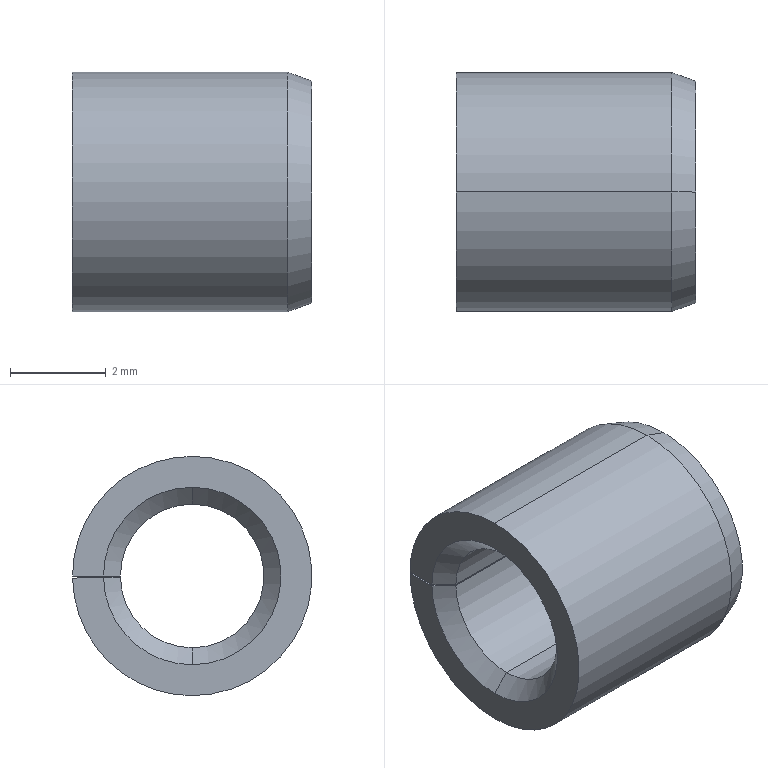Part | SolidWorks | features MBimport 1 | 1 solid | 19 faces | box 5 x 5 x 5 mm | volume 60.695 mm3 | cone 9 | cylinder 6 | plane 4 | commonest cylinder face diameters 3 x3 5 x3
STEP:
#1=CARTESIAN_POINT('',(4.5,0.,2.5));
#2=VERTEX_POINT('',#1);
#3=CARTESIAN_POINT('',(4.5,0.,-2.5));
#4=VERTEX_POINT('',#3);
#5=CARTESIAN_POINT('',(4.5,0.,0.));
#6=DIRECTION('',(1.,0.,0.));
#7=DIRECTION('',(0.,0.,-1.));
#8=AXIS2_PLACEMENT_3D('',#5,#6,#7);
#9=CIRCLE('',#8,2.5);
#10=EDGE_CURVE('',#2,#4,#9,.T.);
#11=ORIENTED_EDGE('',*,*,#10,.F.);
#12=CARTESIAN_POINT('',(0.,0.,2.5));
#13=VERTEX_POINT('',#12);
#14=CARTESIAN_POINT('',(50.,0.,2.5));
#15=DIRECTION('',(-1.,0.,0.));
#16=VECTOR('',#15,1000.);
#17=LINE('',#14,#16);
#18=EDGE_CURVE('',#2,#13,#17,.T.);
#19=ORIENTED_EDGE('',*,*,#18,.T.);
#20=CARTESIAN_POINT('',(0.,0.,-2.5));
#21=VERTEX_POINT('',#20);
#22=CARTESIAN_POINT('',(0.,0.,0.));
#23=DIRECTION('',(1.,0.,0.));
#24=DIRECTION('',(0.,0.,-1.));
#25=AXIS2_PLACEMENT_3D('',#22,#23,#24);
#26=CIRCLE('',#25,2.5);
#27=EDGE_CURVE('',#13,#21,#26,.T.);
#28=ORIENTED_EDGE('',*,*,#27,.T.);
#29=CARTESIAN_POINT('',(50.,0.,-2.5));
#30=DIRECTION('',(-1.,0.,0.));
#31=VECTOR('',#30,1000.);
#32=LINE('',#29,#31);
#33=EDGE_CURVE('',#4,#21,#32,.T.);
#34=ORIENTED_EDGE('',*,*,#33,.F.);
#35=EDGE_LOOP('',(#11,#19,#28,#34));
#36=FACE_OUTER_BOUND('',#35,.T.);
#37=CARTESIAN_POINT('',(50.,0.,0.));
#38=DIRECTION('',(-1.,0.,0.));
#39=DIRECTION('',(0.,0.,-1.));
#40=AXIS2_PLACEMENT_3D('',#37,#38,#39);
#41=CYLINDRICAL_SURFACE('',#40,2.5);
#42=ADVANCED_FACE('',(#36),#41,.T.);
#43=CARTESIAN_POINT('',(4.5,2.5,-0.04363));
#44=VERTEX_POINT('',#43);
#45=CARTESIAN_POINT('',(4.5,0.,0.));
#46=DIRECTION('',(1.,0.,0.));
#47=DIRECTION('',(0.,0.,-1.));
#48=AXIS2_PLACEMENT_3D('',#45,#46,#47);
#49=CIRCLE('',#48,2.5);
#50=EDGE_CURVE('',#4,#44,#49,.T.);
#51=ORIENTED_EDGE('',*,*,#50,.F.);
#52=ORIENTED_EDGE('',*,*,#33,.T.);
#53=CARTESIAN_POINT('',(0.,2.5,-0.04363));
#54=VERTEX_POINT('',#53);
#55=CARTESIAN_POINT('',(0.,0.,0.));
#56=DIRECTION('',(1.,0.,0.));
#57=DIRECTION('',(0.,0.,-1.));
#58=AXIS2_PLACEMENT_3D('',#55,#56,#57);
#59=CIRCLE('',#58,2.5);
#60=EDGE_CURVE('',#21,#54,#59,.T.);
#61=ORIENTED_EDGE('',*,*,#60,.T.);
#62=CARTESIAN_POINT('',(4.5,2.5,-0.04363));
#63=DIRECTION('',(-1.,0.,0.));
#64=VECTOR('',#63,1000.);
#65=LINE('',#62,#64);
#66=EDGE_CURVE('',#44,#54,#65,.T.);
#67=ORIENTED_EDGE('',*,*,#66,.F.);
#68=EDGE_LOOP('',(#51,#52,#61,#67));
#69=FACE_OUTER_BOUND('',#68,.T.);
#70=CARTESIAN_POINT('',(50.,0.,0.));
#71=DIRECTION('',(-1.,0.,0.));
#72=DIRECTION('',(0.,0.,-1.));
#73=AXIS2_PLACEMENT_3D('',#70,#71,#72);
#74=CYLINDRICAL_SURFACE('',#73,2.5);
#75=ADVANCED_FACE('',(#69),#74,.T.);
#76=CARTESIAN_POINT('',(5.,0.,-2.318));
#77=VERTEX_POINT('',#76);
#78=CARTESIAN_POINT('',(5.,2.318,-0.04045));
#79=VERTEX_POINT('',#78);
#80=CARTESIAN_POINT('',(5.,0.,0.));
#81=DIRECTION('',(1.,0.,0.));
#82=DIRECTION('',(0.,0.,-1.));
#83=AXIS2_PLACEMENT_3D('',#80,#81,#82);
#84=CIRCLE('',#83,2.318);
#85=EDGE_CURVE('',#77,#79,#84,.T.);
#86=ORIENTED_EDGE('',*,*,#85,.F.);
#87=CARTESIAN_POINT('',(5.,0.,-2.318));
#88=DIRECTION('',(-0.9397,0.,-0.342));
#89=VECTOR('',#88,1000.);
#90=LINE('',#87,#89);
#91=EDGE_CURVE('',#77,#4,#90,.T.);
#92=ORIENTED_EDGE('',*,*,#91,.T.);
#93=ORIENTED_EDGE('',*,*,#50,.T.);
#94=CARTESIAN_POINT('',(5.,2.318,-0.04045));
#95=DIRECTION('',(-0.9397,0.342,-0.005969));
#96=VECTOR('',#95,1000.);
#97=LINE('',#94,#96);
#98=EDGE_CURVE('',#79,#44,#97,.T.);
#99=ORIENTED_EDGE('',*,*,#98,.F.);
#100=EDGE_LOOP('',(#86,#92,#93,#99));
#101=FACE_OUTER_BOUND('',#100,.T.);
#102=CARTESIAN_POINT('',(5.,0.,0.));
#103=DIRECTION('',(-1.,0.,0.));
#104=DIRECTION('',(0.,0.,1.));
#105=AXIS2_PLACEMENT_3D('',#102,#103,#104);
#106=CONICAL_SURFACE('',#105,2.318,0.3491);
#107=ADVANCED_FACE('',(#101),#106,.T.);
#108=ORIENTED_EDGE('',*,*,#91,.F.);
#109=CARTESIAN_POINT('',(5.,0.,2.318));
#110=VERTEX_POINT('',#109);
#111=CARTESIAN_POINT('',(5.,0.,0.));
#112=DIRECTION('',(1.,0.,0.));
#113=DIRECTION('',(0.,0.,-1.));
#114=AXIS2_PLACEMENT_3D('',#111,#112,#113);
#115=CIRCLE('',#114,2.318);
#116=EDGE_CURVE('',#110,#77,#115,.T.);
#117=ORIENTED_EDGE('',*,*,#116,.F.);
#118=CARTESIAN_POINT('',(5.,0.,2.318));
#119=DIRECTION('',(-0.9397,0.,0.342));
#120=VECTOR('',#119,1000.);
#121=LINE('',#118,#120);
#122=EDGE_CURVE('',#110,#2,#121,.T.);
#123=ORIENTED_EDGE('',*,*,#122,.T.);
#124=ORIENTED_EDGE('',*,*,#10,.T.);
#125=EDGE_LOOP('',(#108,#117,#123,#124));
#126=FACE_OUTER_BOUND('',#125,.T.);
#127=CARTESIAN_POINT('',(5.,0.,0.));
#128=DIRECTION('',(-1.,0.,0.));
#129=DIRECTION('',(0.,0.,1.));
#130=AXIS2_PLACEMENT_3D('',#127,#128,#129);
#131=CONICAL_SURFACE('',#130,2.318,0.3491);
#132=ADVANCED_FACE('',(#126),#131,.T.);
#133=CARTESIAN_POINT('',(0.3536,0.,1.5));
#134=VERTEX_POINT('',#133);
#135=CARTESIAN_POINT('',(0.3536,0.,-1.5));
#136=VERTEX_POINT('',#135);
#137=CARTESIAN_POINT('',(0.3536,0.,0.));
#138=DIRECTION('',(1.,0.,0.));
#139=DIRECTION('',(0.,0.,-1.));
#140=AXIS2_PLACEMENT_3D('',#137,#138,#139);
#141=CIRCLE('',#140,1.5);
#142=EDGE_CURVE('',#134,#136,#141,.T.);
#143=ORIENTED_EDGE('',*,*,#142,.T.);
#144=CARTESIAN_POINT('',(0.,0.,-1.854));
#145=VERTEX_POINT('',#144);
#146=CARTESIAN_POINT('',(0.,0.,-1.854));
#147=DIRECTION('',(-0.7071,0.,-0.7071));
#148=VECTOR('',#147,1000.);
#149=LINE('',#146,#148);
#150=EDGE_CURVE('',#136,#145,#149,.T.);
#151=ORIENTED_EDGE('',*,*,#150,.T.);
#152=CARTESIAN_POINT('',(0.,0.,1.854));
#153=VERTEX_POINT('',#152);
#154=CARTESIAN_POINT('',(0.,0.,0.));
#155=DIRECTION('',(1.,0.,0.));
#156=DIRECTION('',(0.,0.,-1.));
#157=AXIS2_PLACEMENT_3D('',#154,#155,#156);
#158=CIRCLE('',#157,1.854);
#159=EDGE_CURVE('',#153,#145,#158,.T.);
#160=ORIENTED_EDGE('',*,*,#159,.F.);
#161=CARTESIAN_POINT('',(0.,0.,1.854));
#162=DIRECTION('',(-0.7071,0.,0.7071));
#163=VECTOR('',#162,1000.);
#164=LINE('',#161,#163);
#165=EDGE_CURVE('',#134,#153,#164,.T.);
#166=ORIENTED_EDGE('',*,*,#165,.F.);
#167=EDGE_LOOP('',(#143,#151,#160,#166));
#168=FACE_OUTER_BOUND('',#167,.T.);
#169=CARTESIAN_POINT('',(0.,0.,0.));
#170=DIRECTION('',(-1.,0.,0.));
#171=DIRECTION('',(0.,0.,1.));
#172=AXIS2_PLACEMENT_3D('',#169,#170,#171);
#173=CONICAL_SURFACE('',#172,1.854,0.7854);
#174=ADVANCED_FACE('',(#168),#173,.F.);
#175=CARTESIAN_POINT('',(0.3536,1.5,0.));
#176=VERTEX_POINT('',#175);
#177=CARTESIAN_POINT('',(0.3536,0.,0.));
#178=DIRECTION('',(1.,0.,0.));
#179=DIRECTION('',(0.,0.,-1.));
#180=AXIS2_PLACEMENT_3D('',#177,#178,#179);
#181=CIRCLE('',#180,1.5);
#182=EDGE_CURVE('',#176,#134,#181,.T.);
#183=ORIENTED_EDGE('',*,*,#182,.T.);
#184=ORIENTED_EDGE('',*,*,#165,.T.);
#185=CARTESIAN_POINT('',(0.,1.854,0.));
#186=VERTEX_POINT('',#185);
#187=CARTESIAN_POINT('',(0.,0.,0.));
#188=DIRECTION('',(1.,0.,0.));
#189=DIRECTION('',(0.,0.,-1.));
#190=AXIS2_PLACEMENT_3D('',#187,#188,#189);
#191=CIRCLE('',#190,1.854);
#192=EDGE_CURVE('',#186,#153,#191,.T.);
#193=ORIENTED_EDGE('',*,*,#192,.F.);
#194=CARTESIAN_POINT('',(0.,1.854,0.));
#195=DIRECTION('',(0.7071,-0.7071,0.));
#196=VECTOR('',#195,1000.);
#197=LINE('',#194,#196);
#198=EDGE_CURVE('',#186,#176,#197,.T.);
#199=ORIENTED_EDGE('',*,*,#198,.T.);
#200=EDGE_LOOP('',(#183,#184,#193,#199));
#201=FACE_OUTER_BOUND('',#200,.T.);
#202=CARTESIAN_POINT('',(0.,0.,0.));
#203=DIRECTION('',(-1.,0.,0.));
#204=DIRECTION('',(0.,0.,1.));
#205=AXIS2_PLACEMENT_3D('',#202,#203,#204);
#206=CONICAL_SURFACE('',#205,1.854,0.7854);
#207=ADVANCED_FACE('',(#201),#206,.F.);
#208=CARTESIAN_POINT('',(4.646,1.5,0.));
#209=VERTEX_POINT('',#208);
#210=CARTESIAN_POINT('',(4.646,0.,1.5));
#211=VERTEX_POINT('',#210);
#212=CARTESIAN_POINT('',(4.646,0.,0.));
#213=DIRECTION('',(1.,0.,0.));
#214=DIRECTION('',(0.,0.,-1.));
#215=AXIS2_PLACEMENT_3D('',#212,#213,#214);
#216=CIRCLE('',#215,1.5);
#217=EDGE_CURVE('',#209,#211,#216,.T.);
#218=ORIENTED_EDGE('',*,*,#217,.T.);
#219=CARTESIAN_POINT('',(50.,0.,1.5));
#220=DIRECTION('',(-1.,0.,0.));
#221=VECTOR('',#220,1000.);
#222=LINE('',#219,#221);
#223=EDGE_CURVE('',#211,#134,#222,.T.);
#224=ORIENTED_EDGE('',*,*,#223,.T.);
#225=ORIENTED_EDGE('',*,*,#182,.F.);
#226=CARTESIAN_POINT('',(0.3536,1.5,0.));
#227=DIRECTION('',(1.,0.,0.));
#228=VECTOR('',#227,1000.);
#229=LINE('',#226,#228);
#230=EDGE_CURVE('',#176,#209,#229,.T.);
#231=ORIENTED_EDGE('',*,*,#230,.T.);
#232=EDGE_LOOP('',(#218,#224,#225,#231));
#233=FACE_OUTER_BOUND('',#232,.T.);
#234=CARTESIAN_POINT('',(50.,0.,0.));
#235=DIRECTION('',(-1.,0.,0.));
#236=DIRECTION('',(0.,0.,-1.));
#237=AXIS2_PLACEMENT_3D('',#234,#235,#236);
#238=CYLINDRICAL_SURFACE('',#237,1.5);
#239=ADVANCED_FACE('',(#233),#238,.F.);
#240=ORIENTED_EDGE('',*,*,#223,.F.);
#241=CARTESIAN_POINT('',(4.646,0.,-1.5));
#242=VERTEX_POINT('',#241);
#243=CARTESIAN_POINT('',(4.646,0.,0.));
#244=DIRECTION('',(1.,0.,0.));
#245=DIRECTION('',(0.,0.,-1.));
#246=AXIS2_PLACEMENT_3D('',#243,#244,#245);
#247=CIRCLE('',#246,1.5);
#248=EDGE_CURVE('',#211,#242,#247,.T.);
#249=ORIENTED_EDGE('',*,*,#248,.T.);
#250=CARTESIAN_POINT('',(50.,0.,-1.5));
#251=DIRECTION('',(-1.,0.,0.));
#252=VECTOR('',#251,1000.);
#253=LINE('',#250,#252);
#254=EDGE_CURVE('',#242,#136,#253,.T.);
#255=ORIENTED_EDGE('',*,*,#254,.T.);
#256=ORIENTED_EDGE('',*,*,#142,.F.);
#257=EDGE_LOOP('',(#240,#249,#255,#256));
#258=FACE_OUTER_BOUND('',#257,.T.);
#259=CARTESIAN_POINT('',(50.,0.,0.));
#260=DIRECTION('',(-1.,0.,0.));
#261=DIRECTION('',(0.,0.,-1.));
#262=AXIS2_PLACEMENT_3D('',#259,#260,#261);
#263=CYLINDRICAL_SURFACE('',#262,1.5);
#264=ADVANCED_FACE('',(#258),#263,.F.);
#265=ORIENTED_EDGE('',*,*,#248,.F.);
#266=CARTESIAN_POINT('',(5.,0.,1.854));
#267=VERTEX_POINT('',#266);
#268=CARTESIAN_POINT('',(4.646,0.,1.5));
#269=DIRECTION('',(0.7071,0.,0.7071));
#270=VECTOR('',#269,1000.);
#271=LINE('',#268,#270);
#272=EDGE_CURVE('',#211,#267,#271,.T.);
#273=ORIENTED_EDGE('',*,*,#272,.T.);
#274=CARTESIAN_POINT('',(5.,0.,-1.854));
#275=VERTEX_POINT('',#274);
#276=CARTESIAN_POINT('',(5.,0.,0.));
#277=DIRECTION('',(1.,0.,0.));
#278=DIRECTION('',(0.,0.,-1.));
#279=AXIS2_PLACEMENT_3D('',#276,#277,#278);
#280=CIRCLE('',#279,1.854);
#281=EDGE_CURVE('',#267,#275,#280,.T.);
#282=ORIENTED_EDGE('',*,*,#281,.T.);
#283=CARTESIAN_POINT('',(4.646,0.,-1.5));
#284=DIRECTION('',(0.7071,0.,-0.7071));
#285=VECTOR('',#284,1000.);
#286=LINE('',#283,#285);
#287=EDGE_CURVE('',#242,#275,#286,.T.);
#288=ORIENTED_EDGE('',*,*,#287,.F.);
#289=EDGE_LOOP('',(#265,#273,#282,#288));
#290=FACE_OUTER_BOUND('',#289,.T.);
#291=CARTESIAN_POINT('',(4.646,0.,0.));
#292=DIRECTION('',(1.,0.,0.));
#293=DIRECTION('',(0.,0.,-1.));
#294=AXIS2_PLACEMENT_3D('',#291,#292,#293);
#295=CONICAL_SURFACE('',#294,1.5,0.7854);
#296=ADVANCED_FACE('',(#290),#295,.F.);
#297=CARTESIAN_POINT('',(4.646,1.5,-0.02618));
#298=VERTEX_POINT('',#297);
#299=CARTESIAN_POINT('',(4.646,0.,0.));
#300=DIRECTION('',(1.,0.,0.));
#301=DIRECTION('',(0.,0.,-1.));
#302=AXIS2_PLACEMENT_3D('',#299,#300,#301);
#303=CIRCLE('',#302,1.5);
#304=EDGE_CURVE('',#242,#298,#303,.T.);
#305=ORIENTED_EDGE('',*,*,#304,.F.);
#306=ORIENTED_EDGE('',*,*,#287,.T.);
#307=CARTESIAN_POINT('',(5.,1.853,-0.03235));
#308=VERTEX_POINT('',#307);
#309=CARTESIAN_POINT('',(5.,0.,0.));
#310=DIRECTION('',(1.,0.,0.));
#311=DIRECTION('',(0.,0.,-1.));
#312=AXIS2_PLACEMENT_3D('',#309,#310,#311);
#313=CIRCLE('',#312,1.854);
#314=EDGE_CURVE('',#275,#308,#313,.T.);
#315=ORIENTED_EDGE('',*,*,#314,.T.);
#316=CARTESIAN_POINT('',(4.646,1.5,-0.02618));
#317=DIRECTION('',(0.7071,0.707,-0.01234));
#318=VECTOR('',#317,1000.);
#319=LINE('',#316,#318);
#320=EDGE_CURVE('',#298,#308,#319,.T.);
#321=ORIENTED_EDGE('',*,*,#320,.F.);
#322=EDGE_LOOP('',(#305,#306,#315,#321));
#323=FACE_OUTER_BOUND('',#322,.T.);
#324=CARTESIAN_POINT('',(4.646,0.,0.));
#325=DIRECTION('',(1.,0.,0.));
#326=DIRECTION('',(0.,0.,-1.));
#327=AXIS2_PLACEMENT_3D('',#324,#325,#326);
#328=CONICAL_SURFACE('',#327,1.5,0.7854);
#329=ADVANCED_FACE('',(#323),#328,.F.);
#330=CARTESIAN_POINT('',(5.,2.318,0.));
#331=VERTEX_POINT('',#330);
#332=CARTESIAN_POINT('',(5.,0.,0.));
#333=DIRECTION('',(1.,0.,0.));
#334=DIRECTION('',(0.,0.,-1.));
#335=AXIS2_PLACEMENT_3D('',#332,#333,#334);
#336=CIRCLE('',#335,2.318);
#337=EDGE_CURVE('',#331,#110,#336,.T.);
#338=ORIENTED_EDGE('',*,*,#337,.T.);
#339=ORIENTED_EDGE('',*,*,#116,.T.);
#340=ORIENTED_EDGE('',*,*,#85,.T.);
#341=CARTESIAN_POINT('',(5.,1.853,-0.03235));
#342=DIRECTION('',(0.,0.9998,-0.01745));
#343=VECTOR('',#342,1000.);
#344=LINE('',#341,#343);
#345=EDGE_CURVE('',#308,#79,#344,.T.);
#346=ORIENTED_EDGE('',*,*,#345,.F.);
#347=ORIENTED_EDGE('',*,*,#314,.F.);
#348=ORIENTED_EDGE('',*,*,#281,.F.);
#349=CARTESIAN_POINT('',(5.,1.854,0.));
#350=VERTEX_POINT('',#349);
#351=CARTESIAN_POINT('',(5.,0.,0.));
#352=DIRECTION('',(1.,0.,0.));
#353=DIRECTION('',(0.,0.,-1.));
#354=AXIS2_PLACEMENT_3D('',#351,#352,#353);
#355=CIRCLE('',#354,1.854);
#356=EDGE_CURVE('',#350,#267,#355,.T.);
#357=ORIENTED_EDGE('',*,*,#356,.F.);
#358=CARTESIAN_POINT('',(5.,1.854,0.));
#359=DIRECTION('',(0.,1.,0.));
#360=VECTOR('',#359,1000.);
#361=LINE('',#358,#360);
#362=EDGE_CURVE('',#350,#331,#361,.T.);
#363=ORIENTED_EDGE('',*,*,#362,.T.);
#364=EDGE_LOOP('',(#338,#339,#340,#346,#347,#348,#357,#363));
#365=FACE_OUTER_BOUND('',#364,.T.);
#366=CARTESIAN_POINT('',(5.,1.854,0.));
#367=DIRECTION('',(1.,0.,0.));
#368=DIRECTION('',(0.,1.,0.));
#369=AXIS2_PLACEMENT_3D('',#366,#367,#368);
#370=PLANE('',#369);
#371=ADVANCED_FACE('',(#365),#370,.T.);
#372=ORIENTED_EDGE('',*,*,#272,.F.);
#373=ORIENTED_EDGE('',*,*,#217,.F.);
#374=CARTESIAN_POINT('',(4.646,1.5,0.));
#375=DIRECTION('',(0.7071,0.7071,0.));
#376=VECTOR('',#375,1000.);
#377=LINE('',#374,#376);
#378=EDGE_CURVE('',#209,#350,#377,.T.);
#379=ORIENTED_EDGE('',*,*,#378,.T.);
#380=ORIENTED_EDGE('',*,*,#356,.T.);
#381=EDGE_LOOP('',(#372,#373,#379,#380));
#382=FACE_OUTER_BOUND('',#381,.T.);
#383=CARTESIAN_POINT('',(4.646,0.,0.));
#384=DIRECTION('',(1.,0.,0.));
#385=DIRECTION('',(0.,0.,-1.));
#386=AXIS2_PLACEMENT_3D('',#383,#384,#385);
#387=CONICAL_SURFACE('',#386,1.5,0.7854);
#388=ADVANCED_FACE('',(#382),#387,.F.);
#389=ORIENTED_EDGE('',*,*,#254,.F.);
#390=ORIENTED_EDGE('',*,*,#304,.T.);
#391=CARTESIAN_POINT('',(0.3536,1.5,-0.02618));
#392=VERTEX_POINT('',#391);
#393=CARTESIAN_POINT('',(0.3536,1.5,-0.02618));
#394=DIRECTION('',(1.,0.,0.));
#395=VECTOR('',#394,1000.);
#396=LINE('',#393,#395);
#397=EDGE_CURVE('',#392,#298,#396,.T.);
#398=ORIENTED_EDGE('',*,*,#397,.F.);
#399=CARTESIAN_POINT('',(0.3536,0.,0.));
#400=DIRECTION('',(1.,0.,0.));
#401=DIRECTION('',(0.,0.,-1.));
#402=AXIS2_PLACEMENT_3D('',#399,#400,#401);
#403=CIRCLE('',#402,1.5);
#404=EDGE_CURVE('',#136,#392,#403,.T.);
#405=ORIENTED_EDGE('',*,*,#404,.F.);
#406=EDGE_LOOP('',(#389,#390,#398,#405));
#407=FACE_OUTER_BOUND('',#406,.T.);
#408=CARTESIAN_POINT('',(50.,0.,0.));
#409=DIRECTION('',(-1.,0.,0.));
#410=DIRECTION('',(0.,0.,-1.));
#411=AXIS2_PLACEMENT_3D('',#408,#409,#410);
#412=CYLINDRICAL_SURFACE('',#411,1.5);
#413=ADVANCED_FACE('',(#407),#412,.F.);
#414=CARTESIAN_POINT('',(0.,1.853,-0.03235));
#415=VERTEX_POINT('',#414);
#416=CARTESIAN_POINT('',(0.,2.5,-0.04363));
#417=DIRECTION('',(0.,-0.9998,0.01745));
#418=VECTOR('',#417,1000.);
#419=LINE('',#416,#418);
#420=EDGE_CURVE('',#54,#415,#419,.T.);
#421=ORIENTED_EDGE('',*,*,#420,.T.);
#422=CARTESIAN_POINT('',(0.,1.853,-0.03235));
#423=DIRECTION('',(0.7071,-0.707,0.01234));
#424=VECTOR('',#423,1000.);
#425=LINE('',#422,#424);
#426=EDGE_CURVE('',#415,#392,#425,.T.);
#427=ORIENTED_EDGE('',*,*,#426,.T.);
#428=ORIENTED_EDGE('',*,*,#397,.T.);
#429=ORIENTED_EDGE('',*,*,#320,.T.);
#430=ORIENTED_EDGE('',*,*,#345,.T.);
#431=ORIENTED_EDGE('',*,*,#98,.T.);
#432=ORIENTED_EDGE('',*,*,#66,.T.);
#433=EDGE_LOOP('',(#421,#427,#428,#429,#430,#431,#432));
#434=FACE_OUTER_BOUND('',#433,.T.);
#435=CARTESIAN_POINT('',(0.,0.,0.));
#436=DIRECTION('',(0.,0.01745,0.9998));
#437=DIRECTION('',(1.,0.,0.));
#438=AXIS2_PLACEMENT_3D('',#435,#436,#437);
#439=PLANE('',#438);
#440=ADVANCED_FACE('',(#434),#439,.T.);
#441=ORIENTED_EDGE('',*,*,#150,.F.);
#442=ORIENTED_EDGE('',*,*,#404,.T.);
#443=ORIENTED_EDGE('',*,*,#426,.F.);
#444=CARTESIAN_POINT('',(0.,0.,0.));
#445=DIRECTION('',(1.,0.,0.));
#446=DIRECTION('',(0.,0.,-1.));
#447=AXIS2_PLACEMENT_3D('',#444,#445,#446);
#448=CIRCLE('',#447,1.854);
#449=EDGE_CURVE('',#145,#415,#448,.T.);
#450=ORIENTED_EDGE('',*,*,#449,.F.);
#451=EDGE_LOOP('',(#441,#442,#443,#450));
#452=FACE_OUTER_BOUND('',#451,.T.);
#453=CARTESIAN_POINT('',(0.,0.,0.));
#454=DIRECTION('',(-1.,0.,0.));
#455=DIRECTION('',(0.,0.,1.));
#456=AXIS2_PLACEMENT_3D('',#453,#454,#455);
#457=CONICAL_SURFACE('',#456,1.854,0.7854);
#458=ADVANCED_FACE('',(#452),#457,.F.);
#459=ORIENTED_EDGE('',*,*,#192,.T.);
#460=ORIENTED_EDGE('',*,*,#159,.T.);
#461=ORIENTED_EDGE('',*,*,#449,.T.);
#462=ORIENTED_EDGE('',*,*,#420,.F.);
#463=ORIENTED_EDGE('',*,*,#60,.F.);
#464=ORIENTED_EDGE('',*,*,#27,.F.);
#465=CARTESIAN_POINT('',(0.,2.5,0.));
#466=VERTEX_POINT('',#465);
#467=CARTESIAN_POINT('',(0.,0.,0.));
#468=DIRECTION('',(1.,0.,0.));
#469=DIRECTION('',(0.,0.,-1.));
#470=AXIS2_PLACEMENT_3D('',#467,#468,#469);
#471=CIRCLE('',#470,2.5);
#472=EDGE_CURVE('',#466,#13,#471,.T.);
#473=ORIENTED_EDGE('',*,*,#472,.F.);
#474=CARTESIAN_POINT('',(0.,2.5,0.));
#475=DIRECTION('',(0.,-1.,0.));
#476=VECTOR('',#475,1000.);
#477=LINE('',#474,#476);
#478=EDGE_CURVE('',#466,#186,#477,.T.);
#479=ORIENTED_EDGE('',*,*,#478,.T.);
#480=EDGE_LOOP('',(#459,#460,#461,#462,#463,#464,#473,#479));
#481=FACE_OUTER_BOUND('',#480,.T.);
#482=CARTESIAN_POINT('',(0.,2.5,0.));
#483=DIRECTION('',(-1.,0.,0.));
#484=DIRECTION('',(0.,0.,1.));
#485=AXIS2_PLACEMENT_3D('',#482,#483,#484);
#486=PLANE('',#485);
#487=ADVANCED_FACE('',(#481),#486,.T.);
#488=ORIENTED_EDGE('',*,*,#122,.F.);
#489=ORIENTED_EDGE('',*,*,#337,.F.);
#490=CARTESIAN_POINT('',(4.5,2.5,0.));
#491=VERTEX_POINT('',#490);
#492=CARTESIAN_POINT('',(5.,2.318,0.));
#493=DIRECTION('',(-0.9397,0.342,0.));
#494=VECTOR('',#493,1000.);
#495=LINE('',#492,#494);
#496=EDGE_CURVE('',#331,#491,#495,.T.);
#497=ORIENTED_EDGE('',*,*,#496,.T.);
#498=CARTESIAN_POINT('',(4.5,0.,0.));
#499=DIRECTION('',(1.,0.,0.));
#500=DIRECTION('',(0.,0.,-1.));
#501=AXIS2_PLACEMENT_3D('',#498,#499,#500);
#502=CIRCLE('',#501,2.5);
#503=EDGE_CURVE('',#491,#2,#502,.T.);
#504=ORIENTED_EDGE('',*,*,#503,.T.);
#505=EDGE_LOOP('',(#488,#489,#497,#504));
#506=FACE_OUTER_BOUND('',#505,.T.);
#507=CARTESIAN_POINT('',(5.,0.,0.));
#508=DIRECTION('',(-1.,0.,0.));
#509=DIRECTION('',(0.,0.,1.));
#510=AXIS2_PLACEMENT_3D('',#507,#508,#509);
#511=CONICAL_SURFACE('',#510,2.318,0.3491);
#512=ADVANCED_FACE('',(#506),#511,.T.);
#513=ORIENTED_EDGE('',*,*,#478,.F.);
#514=CARTESIAN_POINT('',(4.5,2.5,0.));
#515=DIRECTION('',(-1.,0.,0.));
#516=VECTOR('',#515,1000.);
#517=LINE('',#514,#516);
#518=EDGE_CURVE('',#491,#466,#517,.T.);
#519=ORIENTED_EDGE('',*,*,#518,.F.);
#520=ORIENTED_EDGE('',*,*,#496,.F.);
#521=ORIENTED_EDGE('',*,*,#362,.F.);
#522=ORIENTED_EDGE('',*,*,#378,.F.);
#523=ORIENTED_EDGE('',*,*,#230,.F.);
#524=ORIENTED_EDGE('',*,*,#198,.F.);
#525=EDGE_LOOP('',(#513,#519,#520,#521,#522,#523,#524));
#526=FACE_OUTER_BOUND('',#525,.T.);
#527=CARTESIAN_POINT('',(0.,0.,0.));
#528=DIRECTION('',(0.,0.,1.));
#529=DIRECTION('',(0.,-1.,0.));
#530=AXIS2_PLACEMENT_3D('',#527,#528,#529);
#531=PLANE('',#530);
#532=ADVANCED_FACE('',(#526),#531,.F.);
#533=ORIENTED_EDGE('',*,*,#18,.F.);
#534=ORIENTED_EDGE('',*,*,#503,.F.);
#535=ORIENTED_EDGE('',*,*,#518,.T.);
#536=ORIENTED_EDGE('',*,*,#472,.T.);
#537=EDGE_LOOP('',(#533,#534,#535,#536));
#538=FACE_OUTER_BOUND('',#537,.T.);
#539=CARTESIAN_POINT('',(50.,0.,0.));
#540=DIRECTION('',(-1.,0.,0.));
#541=DIRECTION('',(0.,0.,-1.));
#542=AXIS2_PLACEMENT_3D('',#539,#540,#541);
#543=CYLINDRICAL_SURFACE('',#542,2.5);
#544=ADVANCED_FACE('',(#538),#543,.T.);
#545=CLOSED_SHELL('',(#42,#75,#107,#132,#174,#207,#239,#264,#296,#329,#371,#388,#413,#440,#458,#487,#512,#532,#544));
#546=MANIFOLD_SOLID_BREP('',#545);
#547=CARTESIAN_POINT('',(0.,0.,0.));
#548=DIRECTION('',(0.,0.,1.));
#549=DIRECTION('',(1.,0.,0.));
#550=AXIS2_PLACEMENT_3D('',#547,#548,#549);
#551=(LENGTH_UNIT()NAMED_UNIT(*)SI_UNIT(.MILLI.,.METRE.));
#552=UNCERTAINTY_MEASURE_WITH_UNIT(LENGTH_MEASURE(0.00001),#551,'','');
#553=(NAMED_UNIT(*)PLANE_ANGLE_UNIT()SI_UNIT($,.RADIAN.));
#554=(NAMED_UNIT(*)SI_UNIT($,.STERADIAN.)SOLID_ANGLE_UNIT());
#555=(GEOMETRIC_REPRESENTATION_CONTEXT(3)GLOBAL_UNCERTAINTY_ASSIGNED_CONTEXT((#552))GLOBAL_UNIT_ASSIGNED_CONTEXT((#551,#553,#554))REPRESENTATION_CONTEXT('',''));
#556=ADVANCED_BREP_SHAPE_REPRESENTATION('',(#546,#550),#555);